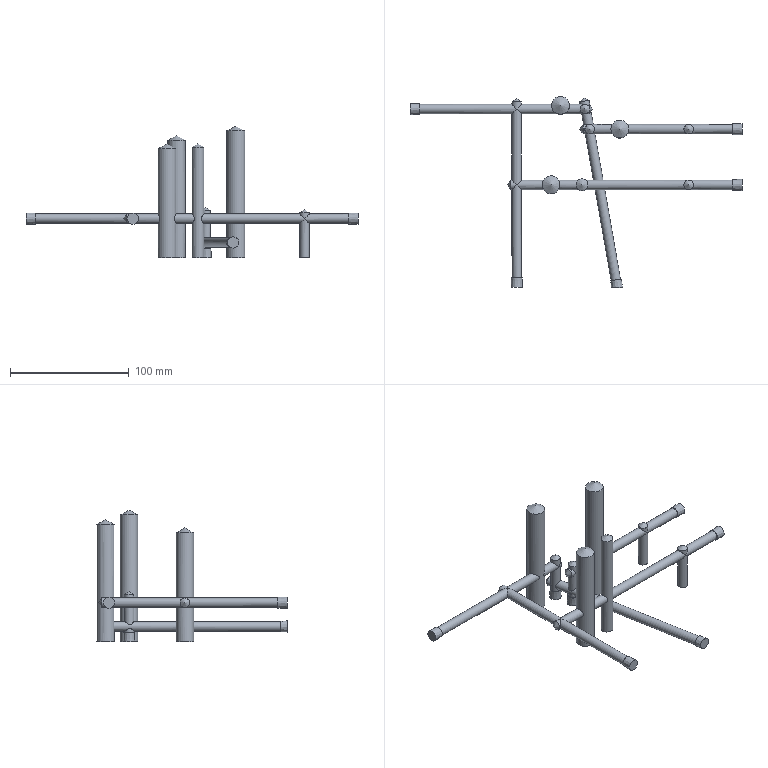Part | STEP file | 车灯-后视镜_id518_x_t | 1 solid | 70 faces | box 280 x 161 x 111 mm | volume 104739 mm3 | cylinder 30 | plane 20 | cone 20 | commonest cylinder face diameters 8 x26 15 x3 10 x1